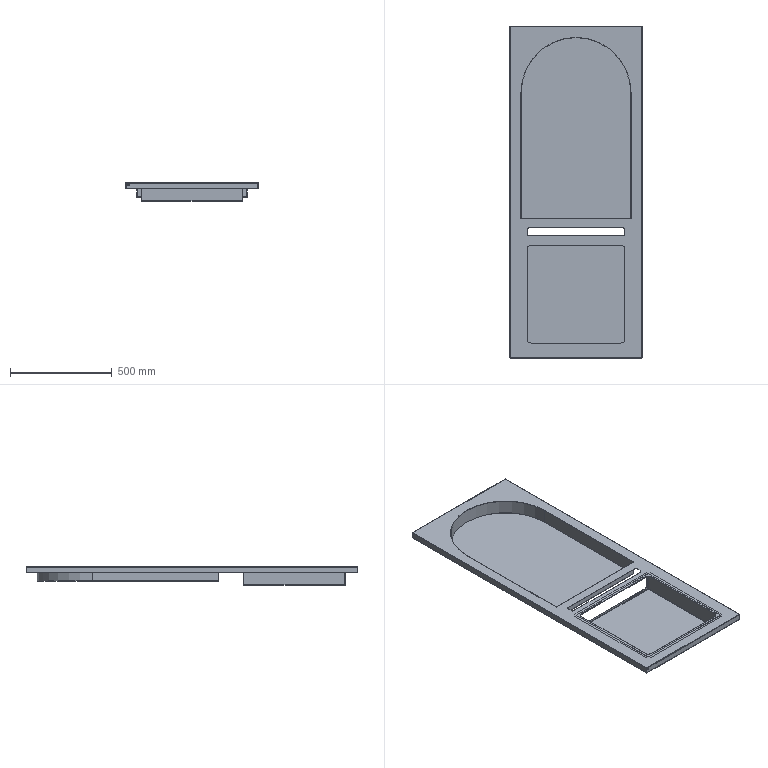Part | SolidWorks | 3 solids | 207 faces | box 648 x 1628 x 92.4 mm | volume 1922415 mm3 | plane 140 | cylinder 51 | spline 16 | commonest cylinder face diameters 2 x16 4.4 x16 20 x8 8 x4 40 x4 540 x2